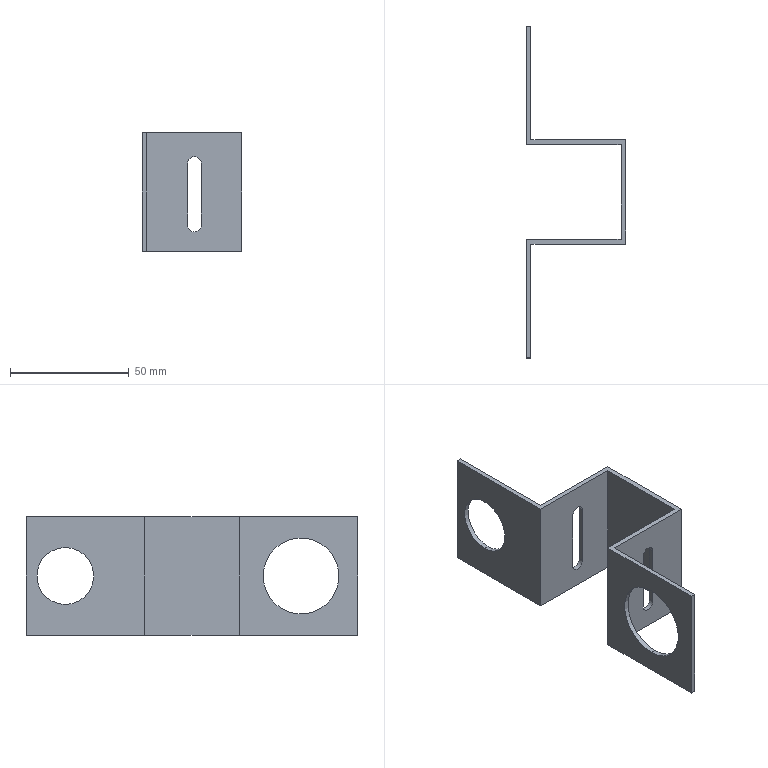Part | SolidWorks | features ICE 3, Extrusion 1 | 1 solid | 28 faces | box 42 x 140 x 50 mm | volume 18778 mm3 | plane 18 | cylinder 10 | commonest cylinder face diameters 5.797 x6 24 x2 32 x2
STEP:
#1=CARTESIAN_POINT('',(0.,33.474,37.));
#2=VERTEX_POINT('',#1);
#3=CARTESIAN_POINT('',(0.,33.474,13.));
#4=VERTEX_POINT('',#3);
#5=CARTESIAN_POINT('',(0.,33.474,25.));
#6=DIRECTION('',(1.,0.,0.));
#7=DIRECTION('',(0.,1.,0.));
#8=AXIS2_PLACEMENT_3D('',#5,#6,#7);
#9=CIRCLE('',#8,12.);
#10=EDGE_CURVE('',#2,#4,#9,.T.);
#11=ORIENTED_EDGE('',*,*,#10,.F.);
#12=CARTESIAN_POINT('',(2.,33.474,37.));
#13=VERTEX_POINT('',#12);
#14=CARTESIAN_POINT('',(-48.,33.474,37.));
#15=DIRECTION('',(1.,0.,0.));
#16=VECTOR('',#15,1000.);
#17=LINE('',#14,#16);
#18=EDGE_CURVE('',#2,#13,#17,.T.);
#19=ORIENTED_EDGE('',*,*,#18,.T.);
#20=CARTESIAN_POINT('',(2.,33.474,13.));
#21=VERTEX_POINT('',#20);
#22=CARTESIAN_POINT('',(2.,33.474,25.));
#23=DIRECTION('',(1.,0.,0.));
#24=DIRECTION('',(0.,0.,-1.));
#25=AXIS2_PLACEMENT_3D('',#22,#23,#24);
#26=CIRCLE('',#25,12.);
#27=EDGE_CURVE('',#13,#21,#26,.T.);
#28=ORIENTED_EDGE('',*,*,#27,.T.);
#29=CARTESIAN_POINT('',(-48.,33.474,13.));
#30=DIRECTION('',(1.,0.,0.));
#31=VECTOR('',#30,1000.);
#32=LINE('',#29,#31);
#33=EDGE_CURVE('',#4,#21,#32,.T.);
#34=ORIENTED_EDGE('',*,*,#33,.F.);
#35=EDGE_LOOP('',(#11,#19,#28,#34));
#36=FACE_OUTER_BOUND('',#35,.T.);
#37=CARTESIAN_POINT('',(-48.,33.474,25.));
#38=DIRECTION('',(1.,0.,0.));
#39=DIRECTION('',(0.,0.,-1.));
#40=AXIS2_PLACEMENT_3D('',#37,#38,#39);
#41=CYLINDRICAL_SURFACE('',#40,12.);
#42=ADVANCED_FACE('',(#36),#41,.F.);
#43=CARTESIAN_POINT('',(0.,-66.,41.));
#44=VERTEX_POINT('',#43);
#45=CARTESIAN_POINT('',(0.,-66.,9.));
#46=VERTEX_POINT('',#45);
#47=CARTESIAN_POINT('',(0.,-66.,25.));
#48=DIRECTION('',(1.,0.,0.));
#49=DIRECTION('',(0.,1.,0.));
#50=AXIS2_PLACEMENT_3D('',#47,#48,#49);
#51=CIRCLE('',#50,16.);
#52=EDGE_CURVE('',#44,#46,#51,.T.);
#53=ORIENTED_EDGE('',*,*,#52,.F.);
#54=CARTESIAN_POINT('',(2.,-66.,41.));
#55=VERTEX_POINT('',#54);
#56=CARTESIAN_POINT('',(-48.,-66.,41.));
#57=DIRECTION('',(1.,0.,0.));
#58=VECTOR('',#57,1000.);
#59=LINE('',#56,#58);
#60=EDGE_CURVE('',#44,#55,#59,.T.);
#61=ORIENTED_EDGE('',*,*,#60,.T.);
#62=CARTESIAN_POINT('',(2.,-66.,9.));
#63=VERTEX_POINT('',#62);
#64=CARTESIAN_POINT('',(2.,-66.,25.));
#65=DIRECTION('',(1.,0.,0.));
#66=DIRECTION('',(0.,0.,-1.));
#67=AXIS2_PLACEMENT_3D('',#64,#65,#66);
#68=CIRCLE('',#67,16.);
#69=EDGE_CURVE('',#55,#63,#68,.T.);
#70=ORIENTED_EDGE('',*,*,#69,.T.);
#71=CARTESIAN_POINT('',(-48.,-66.,9.));
#72=DIRECTION('',(1.,0.,0.));
#73=VECTOR('',#72,1000.);
#74=LINE('',#71,#73);
#75=EDGE_CURVE('',#46,#63,#74,.T.);
#76=ORIENTED_EDGE('',*,*,#75,.F.);
#77=EDGE_LOOP('',(#53,#61,#70,#76));
#78=FACE_OUTER_BOUND('',#77,.T.);
#79=CARTESIAN_POINT('',(-48.,-66.,25.));
#80=DIRECTION('',(1.,0.,0.));
#81=DIRECTION('',(0.,0.,-1.));
#82=AXIS2_PLACEMENT_3D('',#79,#80,#81);
#83=CYLINDRICAL_SURFACE('',#82,16.);
#84=ADVANCED_FACE('',(#78),#83,.F.);
#85=CARTESIAN_POINT('',(22.,-42.,39.928));
#86=VERTEX_POINT('',#85);
#87=CARTESIAN_POINT('',(24.898,-42.,37.029));
#88=VERTEX_POINT('',#87);
#89=CARTESIAN_POINT('',(22.,-42.,37.029));
#90=DIRECTION('',(0.,1.,0.));
#91=DIRECTION('',(0.,0.,1.));
#92=AXIS2_PLACEMENT_3D('',#89,#90,#91);
#93=CIRCLE('',#92,2.898);
#94=EDGE_CURVE('',#86,#88,#93,.T.);
#95=ORIENTED_EDGE('',*,*,#94,.F.);
#96=CARTESIAN_POINT('',(22.,-40.,39.928));
#97=VERTEX_POINT('',#96);
#98=CARTESIAN_POINT('',(22.,-48.,39.928));
#99=DIRECTION('',(0.,1.,0.));
#100=VECTOR('',#99,1000.);
#101=LINE('',#98,#100);
#102=EDGE_CURVE('',#86,#97,#101,.T.);
#103=ORIENTED_EDGE('',*,*,#102,.T.);
#104=CARTESIAN_POINT('',(24.898,-40.,37.029));
#105=VERTEX_POINT('',#104);
#106=CARTESIAN_POINT('',(22.,-40.,37.029));
#107=DIRECTION('',(0.,-1.,0.));
#108=DIRECTION('',(1.,0.,0.));
#109=AXIS2_PLACEMENT_3D('',#106,#107,#108);
#110=CIRCLE('',#109,2.898);
#111=EDGE_CURVE('',#105,#97,#110,.T.);
#112=ORIENTED_EDGE('',*,*,#111,.F.);
#113=CARTESIAN_POINT('',(24.898,-48.,37.029));
#114=DIRECTION('',(0.,1.,0.));
#115=VECTOR('',#114,1000.);
#116=LINE('',#113,#115);
#117=EDGE_CURVE('',#88,#105,#116,.T.);
#118=ORIENTED_EDGE('',*,*,#117,.F.);
#119=EDGE_LOOP('',(#95,#103,#112,#118));
#120=FACE_OUTER_BOUND('',#119,.T.);
#121=CARTESIAN_POINT('',(22.,-48.,37.029));
#122=DIRECTION('',(0.,1.,0.));
#123=DIRECTION('',(0.,0.,1.));
#124=AXIS2_PLACEMENT_3D('',#121,#122,#123);
#125=CYLINDRICAL_SURFACE('',#124,2.898);
#126=ADVANCED_FACE('',(#120),#125,.F.);
#127=CARTESIAN_POINT('',(22.,0.,39.928));
#128=VERTEX_POINT('',#127);
#129=CARTESIAN_POINT('',(24.898,0.,37.029));
#130=VERTEX_POINT('',#129);
#131=CARTESIAN_POINT('',(22.,0.,37.029));
#132=DIRECTION('',(0.,1.,0.));
#133=DIRECTION('',(0.,0.,1.));
#134=AXIS2_PLACEMENT_3D('',#131,#132,#133);
#135=CIRCLE('',#134,2.898);
#136=EDGE_CURVE('',#128,#130,#135,.T.);
#137=ORIENTED_EDGE('',*,*,#136,.F.);
#138=CARTESIAN_POINT('',(22.,2.,39.928));
#139=VERTEX_POINT('',#138);
#140=CARTESIAN_POINT('',(22.,-48.,39.928));
#141=DIRECTION('',(0.,1.,0.));
#142=VECTOR('',#141,1000.);
#143=LINE('',#140,#142);
#144=EDGE_CURVE('',#128,#139,#143,.T.);
#145=ORIENTED_EDGE('',*,*,#144,.T.);
#146=CARTESIAN_POINT('',(24.898,2.,37.029));
#147=VERTEX_POINT('',#146);
#148=CARTESIAN_POINT('',(22.,2.,37.029));
#149=DIRECTION('',(0.,1.,0.));
#150=DIRECTION('',(0.,0.,1.));
#151=AXIS2_PLACEMENT_3D('',#148,#149,#150);
#152=CIRCLE('',#151,2.898);
#153=EDGE_CURVE('',#139,#147,#152,.T.);
#154=ORIENTED_EDGE('',*,*,#153,.T.);
#155=CARTESIAN_POINT('',(24.898,-48.,37.029));
#156=DIRECTION('',(0.,1.,0.));
#157=VECTOR('',#156,1000.);
#158=LINE('',#155,#157);
#159=EDGE_CURVE('',#130,#147,#158,.T.);
#160=ORIENTED_EDGE('',*,*,#159,.F.);
#161=EDGE_LOOP('',(#137,#145,#154,#160));
#162=FACE_OUTER_BOUND('',#161,.T.);
#163=CARTESIAN_POINT('',(22.,-48.,37.029));
#164=DIRECTION('',(0.,1.,0.));
#165=DIRECTION('',(0.,0.,1.));
#166=AXIS2_PLACEMENT_3D('',#163,#164,#165);
#167=CYLINDRICAL_SURFACE('',#166,2.898);
#168=ADVANCED_FACE('',(#162),#167,.F.);
#169=CARTESIAN_POINT('',(2.,50.,0.));
#170=VERTEX_POINT('',#169);
#171=CARTESIAN_POINT('',(0.,50.,0.));
#172=VERTEX_POINT('',#171);
#173=CARTESIAN_POINT('',(0.,50.,0.));
#174=DIRECTION('',(-1.,0.,0.));
#175=VECTOR('',#174,1000.);
#176=LINE('',#173,#175);
#177=EDGE_CURVE('',#170,#172,#176,.T.);
#178=ORIENTED_EDGE('',*,*,#177,.T.);
#179=CARTESIAN_POINT('',(0.,50.,50.));
#180=VERTEX_POINT('',#179);
#181=CARTESIAN_POINT('',(0.,50.,50.));
#182=DIRECTION('',(0.,0.,-1.));
#183=VECTOR('',#182,1000.);
#184=LINE('',#181,#183);
#185=EDGE_CURVE('',#180,#172,#184,.T.);
#186=ORIENTED_EDGE('',*,*,#185,.F.);
#187=CARTESIAN_POINT('',(2.,50.,50.));
#188=VERTEX_POINT('',#187);
#189=CARTESIAN_POINT('',(0.,50.,50.));
#190=DIRECTION('',(-1.,0.,0.));
#191=VECTOR('',#190,1000.);
#192=LINE('',#189,#191);
#193=EDGE_CURVE('',#188,#180,#192,.T.);
#194=ORIENTED_EDGE('',*,*,#193,.F.);
#195=CARTESIAN_POINT('',(2.,50.,50.));
#196=DIRECTION('',(0.,0.,-1.));
#197=VECTOR('',#196,1000.);
#198=LINE('',#195,#197);
#199=EDGE_CURVE('',#188,#170,#198,.T.);
#200=ORIENTED_EDGE('',*,*,#199,.T.);
#201=EDGE_LOOP('',(#178,#186,#194,#200));
#202=FACE_OUTER_BOUND('',#201,.T.);
#203=CARTESIAN_POINT('',(0.,50.,50.));
#204=DIRECTION('',(0.,-1.,0.));
#205=DIRECTION('',(0.,0.,-1.));
#206=AXIS2_PLACEMENT_3D('',#203,#204,#205);
#207=PLANE('',#206);
#208=ADVANCED_FACE('',(#202),#207,.F.);
#209=CARTESIAN_POINT('',(0.,33.474,25.));
#210=DIRECTION('',(1.,0.,0.));
#211=DIRECTION('',(0.,1.,0.));
#212=AXIS2_PLACEMENT_3D('',#209,#210,#211);
#213=CIRCLE('',#212,12.);
#214=EDGE_CURVE('',#4,#2,#213,.T.);
#215=ORIENTED_EDGE('',*,*,#214,.T.);
#216=ORIENTED_EDGE('',*,*,#10,.T.);
#217=EDGE_LOOP('',(#215,#216));
#218=FACE_BOUND('',#217,.T.);
#219=CARTESIAN_POINT('',(0.,0.,0.));
#220=VERTEX_POINT('',#219);
#221=CARTESIAN_POINT('',(0.,50.,0.));
#222=DIRECTION('',(0.,-1.,0.));
#223=VECTOR('',#222,1000.);
#224=LINE('',#221,#223);
#225=EDGE_CURVE('',#172,#220,#224,.T.);
#226=ORIENTED_EDGE('',*,*,#225,.T.);
#227=CARTESIAN_POINT('',(0.,0.,50.));
#228=VERTEX_POINT('',#227);
#229=CARTESIAN_POINT('',(0.,0.,50.));
#230=DIRECTION('',(0.,0.,-1.));
#231=VECTOR('',#230,1000.);
#232=LINE('',#229,#231);
#233=EDGE_CURVE('',#228,#220,#232,.T.);
#234=ORIENTED_EDGE('',*,*,#233,.F.);
#235=CARTESIAN_POINT('',(0.,50.,50.));
#236=DIRECTION('',(0.,-1.,0.));
#237=VECTOR('',#236,1000.);
#238=LINE('',#235,#237);
#239=EDGE_CURVE('',#180,#228,#238,.T.);
#240=ORIENTED_EDGE('',*,*,#239,.F.);
#241=ORIENTED_EDGE('',*,*,#185,.T.);
#242=EDGE_LOOP('',(#226,#234,#240,#241));
#243=FACE_OUTER_BOUND('',#242,.T.);
#244=CARTESIAN_POINT('',(0.,50.,50.));
#245=DIRECTION('',(1.,0.,0.));
#246=DIRECTION('',(0.,1.,0.));
#247=AXIS2_PLACEMENT_3D('',#244,#245,#246);
#248=PLANE('',#247);
#249=ADVANCED_FACE('',(#218,#243),#248,.F.);
#250=CARTESIAN_POINT('',(24.898,0.,11.027));
#251=VERTEX_POINT('',#250);
#252=CARTESIAN_POINT('',(24.898,0.,50.));
#253=DIRECTION('',(0.,0.,-1.));
#254=VECTOR('',#253,1000.);
#255=LINE('',#252,#254);
#256=EDGE_CURVE('',#130,#251,#255,.T.);
#257=ORIENTED_EDGE('',*,*,#256,.T.);
#258=CARTESIAN_POINT('',(19.102,0.,11.027));
#259=VERTEX_POINT('',#258);
#260=CARTESIAN_POINT('',(22.,0.,11.027));
#261=DIRECTION('',(0.,1.,0.));
#262=DIRECTION('',(0.,0.,1.));
#263=AXIS2_PLACEMENT_3D('',#260,#261,#262);
#264=CIRCLE('',#263,2.898);
#265=EDGE_CURVE('',#251,#259,#264,.T.);
#266=ORIENTED_EDGE('',*,*,#265,.T.);
#267=CARTESIAN_POINT('',(19.102,0.,37.029));
#268=VERTEX_POINT('',#267);
#269=CARTESIAN_POINT('',(19.102,0.,50.));
#270=DIRECTION('',(0.,0.,1.));
#271=VECTOR('',#270,1000.);
#272=LINE('',#269,#271);
#273=EDGE_CURVE('',#259,#268,#272,.T.);
#274=ORIENTED_EDGE('',*,*,#273,.T.);
#275=CARTESIAN_POINT('',(22.,0.,37.029));
#276=DIRECTION('',(0.,1.,0.));
#277=DIRECTION('',(0.,0.,1.));
#278=AXIS2_PLACEMENT_3D('',#275,#276,#277);
#279=CIRCLE('',#278,2.898);
#280=EDGE_CURVE('',#268,#128,#279,.T.);
#281=ORIENTED_EDGE('',*,*,#280,.T.);
#282=ORIENTED_EDGE('',*,*,#136,.T.);
#283=EDGE_LOOP('',(#257,#266,#274,#281,#282));
#284=FACE_BOUND('',#283,.T.);
#285=CARTESIAN_POINT('',(40.,0.,0.));
#286=VERTEX_POINT('',#285);
#287=CARTESIAN_POINT('',(0.,0.,0.));
#288=DIRECTION('',(1.,0.,0.));
#289=VECTOR('',#288,1000.);
#290=LINE('',#287,#289);
#291=EDGE_CURVE('',#220,#286,#290,.T.);
#292=ORIENTED_EDGE('',*,*,#291,.T.);
#293=CARTESIAN_POINT('',(40.,0.,50.));
#294=VERTEX_POINT('',#293);
#295=CARTESIAN_POINT('',(40.,0.,50.));
#296=DIRECTION('',(0.,0.,-1.));
#297=VECTOR('',#296,1000.);
#298=LINE('',#295,#297);
#299=EDGE_CURVE('',#294,#286,#298,.T.);
#300=ORIENTED_EDGE('',*,*,#299,.F.);
#301=CARTESIAN_POINT('',(0.,0.,50.));
#302=DIRECTION('',(1.,0.,0.));
#303=VECTOR('',#302,1000.);
#304=LINE('',#301,#303);
#305=EDGE_CURVE('',#228,#294,#304,.T.);
#306=ORIENTED_EDGE('',*,*,#305,.F.);
#307=ORIENTED_EDGE('',*,*,#233,.T.);
#308=EDGE_LOOP('',(#292,#300,#306,#307));
#309=FACE_OUTER_BOUND('',#308,.T.);
#310=CARTESIAN_POINT('',(0.,0.,50.));
#311=DIRECTION('',(0.,1.,0.));
#312=DIRECTION('',(0.,0.,1.));
#313=AXIS2_PLACEMENT_3D('',#310,#311,#312);
#314=PLANE('',#313);
#315=ADVANCED_FACE('',(#284,#309),#314,.F.);
#316=CARTESIAN_POINT('',(40.,-40.,0.));
#317=VERTEX_POINT('',#316);
#318=CARTESIAN_POINT('',(40.,0.,0.));
#319=DIRECTION('',(0.,-1.,0.));
#320=VECTOR('',#319,1000.);
#321=LINE('',#318,#320);
#322=EDGE_CURVE('',#286,#317,#321,.T.);
#323=ORIENTED_EDGE('',*,*,#322,.T.);
#324=CARTESIAN_POINT('',(40.,-40.,50.));
#325=VERTEX_POINT('',#324);
#326=CARTESIAN_POINT('',(40.,-40.,50.));
#327=DIRECTION('',(0.,0.,-1.));
#328=VECTOR('',#327,1000.);
#329=LINE('',#326,#328);
#330=EDGE_CURVE('',#325,#317,#329,.T.);
#331=ORIENTED_EDGE('',*,*,#330,.F.);
#332=CARTESIAN_POINT('',(40.,0.,50.));
#333=DIRECTION('',(0.,-1.,0.));
#334=VECTOR('',#333,1000.);
#335=LINE('',#332,#334);
#336=EDGE_CURVE('',#294,#325,#335,.T.);
#337=ORIENTED_EDGE('',*,*,#336,.F.);
#338=ORIENTED_EDGE('',*,*,#299,.T.);
#339=EDGE_LOOP('',(#323,#331,#337,#338));
#340=FACE_OUTER_BOUND('',#339,.T.);
#341=CARTESIAN_POINT('',(40.,0.,50.));
#342=DIRECTION('',(1.,0.,0.));
#343=DIRECTION('',(0.,0.,-1.));
#344=AXIS2_PLACEMENT_3D('',#341,#342,#343);
#345=PLANE('',#344);
#346=ADVANCED_FACE('',(#340),#345,.F.);
#347=CARTESIAN_POINT('',(19.102,-40.,37.029));
#348=VERTEX_POINT('',#347);
#349=CARTESIAN_POINT('',(19.102,-40.,11.027));
#350=VERTEX_POINT('',#349);
#351=CARTESIAN_POINT('',(19.102,-40.,50.));
#352=DIRECTION('',(0.,0.,-1.));
#353=VECTOR('',#352,1000.);
#354=LINE('',#351,#353);
#355=EDGE_CURVE('',#348,#350,#354,.T.);
#356=ORIENTED_EDGE('',*,*,#355,.T.);
#357=CARTESIAN_POINT('',(24.898,-40.,11.027));
#358=VERTEX_POINT('',#357);
#359=CARTESIAN_POINT('',(22.,-40.,11.027));
#360=DIRECTION('',(0.,-1.,0.));
#361=DIRECTION('',(1.,0.,0.));
#362=AXIS2_PLACEMENT_3D('',#359,#360,#361);
#363=CIRCLE('',#362,2.898);
#364=EDGE_CURVE('',#350,#358,#363,.T.);
#365=ORIENTED_EDGE('',*,*,#364,.T.);
#366=CARTESIAN_POINT('',(24.898,-40.,50.));
#367=DIRECTION('',(0.,0.,1.));
#368=VECTOR('',#367,1000.);
#369=LINE('',#366,#368);
#370=EDGE_CURVE('',#358,#105,#369,.T.);
#371=ORIENTED_EDGE('',*,*,#370,.T.);
#372=ORIENTED_EDGE('',*,*,#111,.T.);
#373=CARTESIAN_POINT('',(22.,-40.,37.029));
#374=DIRECTION('',(0.,-1.,0.));
#375=DIRECTION('',(1.,0.,0.));
#376=AXIS2_PLACEMENT_3D('',#373,#374,#375);
#377=CIRCLE('',#376,2.898);
#378=EDGE_CURVE('',#97,#348,#377,.T.);
#379=ORIENTED_EDGE('',*,*,#378,.T.);
#380=EDGE_LOOP('',(#356,#365,#371,#372,#379));
#381=FACE_BOUND('',#380,.T.);
#382=CARTESIAN_POINT('',(0.,-40.,0.));
#383=VERTEX_POINT('',#382);
#384=CARTESIAN_POINT('',(40.,-40.,0.));
#385=DIRECTION('',(-1.,0.,0.));
#386=VECTOR('',#385,1000.);
#387=LINE('',#384,#386);
#388=EDGE_CURVE('',#317,#383,#387,.T.);
#389=ORIENTED_EDGE('',*,*,#388,.T.);
#390=CARTESIAN_POINT('',(0.,-40.,50.));
#391=VERTEX_POINT('',#390);
#392=CARTESIAN_POINT('',(0.,-40.,50.));
#393=DIRECTION('',(0.,0.,-1.));
#394=VECTOR('',#393,1000.);
#395=LINE('',#392,#394);
#396=EDGE_CURVE('',#391,#383,#395,.T.);
#397=ORIENTED_EDGE('',*,*,#396,.F.);
#398=CARTESIAN_POINT('',(40.,-40.,50.));
#399=DIRECTION('',(-1.,0.,0.));
#400=VECTOR('',#399,1000.);
#401=LINE('',#398,#400);
#402=EDGE_CURVE('',#325,#391,#401,.T.);
#403=ORIENTED_EDGE('',*,*,#402,.F.);
#404=ORIENTED_EDGE('',*,*,#330,.T.);
#405=EDGE_LOOP('',(#389,#397,#403,#404));
#406=FACE_OUTER_BOUND('',#405,.T.);
#407=CARTESIAN_POINT('',(40.,-40.,50.));
#408=DIRECTION('',(0.,-1.,0.));
#409=DIRECTION('',(1.,0.,0.));
#410=AXIS2_PLACEMENT_3D('',#407,#408,#409);
#411=PLANE('',#410);
#412=ADVANCED_FACE('',(#381,#406),#411,.F.);
#413=CARTESIAN_POINT('',(0.,-66.,25.));
#414=DIRECTION('',(1.,0.,0.));
#415=DIRECTION('',(0.,1.,0.));
#416=AXIS2_PLACEMENT_3D('',#413,#414,#415);
#417=CIRCLE('',#416,16.);
#418=EDGE_CURVE('',#46,#44,#417,.T.);
#419=ORIENTED_EDGE('',*,*,#418,.T.);
#420=ORIENTED_EDGE('',*,*,#52,.T.);
#421=EDGE_LOOP('',(#419,#420));
#422=FACE_BOUND('',#421,.T.);
#423=CARTESIAN_POINT('',(0.,-90.,0.));
#424=VERTEX_POINT('',#423);
#425=CARTESIAN_POINT('',(0.,-40.,0.));
#426=DIRECTION('',(0.,-1.,0.));
#427=VECTOR('',#426,1000.);
#428=LINE('',#425,#427);
#429=EDGE_CURVE('',#383,#424,#428,.T.);
#430=ORIENTED_EDGE('',*,*,#429,.T.);
#431=CARTESIAN_POINT('',(0.,-90.,50.));
#432=VERTEX_POINT('',#431);
#433=CARTESIAN_POINT('',(0.,-90.,50.));
#434=DIRECTION('',(0.,0.,-1.));
#435=VECTOR('',#434,1000.);
#436=LINE('',#433,#435);
#437=EDGE_CURVE('',#432,#424,#436,.T.);
#438=ORIENTED_EDGE('',*,*,#437,.F.);
#439=CARTESIAN_POINT('',(0.,-40.,50.));
#440=DIRECTION('',(0.,-1.,0.));
#441=VECTOR('',#440,1000.);
#442=LINE('',#439,#441);
#443=EDGE_CURVE('',#391,#432,#442,.T.);
#444=ORIENTED_EDGE('',*,*,#443,.F.);
#445=ORIENTED_EDGE('',*,*,#396,.T.);
#446=EDGE_LOOP('',(#430,#438,#444,#445));
#447=FACE_OUTER_BOUND('',#446,.T.);
#448=CARTESIAN_POINT('',(0.,-40.,50.));
#449=DIRECTION('',(1.,0.,0.));
#450=DIRECTION('',(0.,1.,0.));
#451=AXIS2_PLACEMENT_3D('',#448,#449,#450);
#452=PLANE('',#451);
#453=ADVANCED_FACE('',(#422,#447),#452,.F.);
#454=CARTESIAN_POINT('',(2.,-90.,0.));
#455=VERTEX_POINT('',#454);
#456=CARTESIAN_POINT('',(0.,-90.,0.));
#457=DIRECTION('',(1.,0.,0.));
#458=VECTOR('',#457,1000.);
#459=LINE('',#456,#458);
#460=EDGE_CURVE('',#424,#455,#459,.T.);
#461=ORIENTED_EDGE('',*,*,#460,.T.);
#462=CARTESIAN_POINT('',(2.,-90.,50.));
#463=VERTEX_POINT('',#462);
#464=CARTESIAN_POINT('',(2.,-90.,50.));
#465=DIRECTION('',(0.,0.,-1.));
#466=VECTOR('',#465,1000.);
#467=LINE('',#464,#466);
#468=EDGE_CURVE('',#463,#455,#467,.T.);
#469=ORIENTED_EDGE('',*,*,#468,.F.);
#470=CARTESIAN_POINT('',(0.,-90.,50.));
#471=DIRECTION('',(1.,0.,0.));
#472=VECTOR('',#471,1000.);
#473=LINE('',#470,#472);
#474=EDGE_CURVE('',#432,#463,#473,.T.);
#475=ORIENTED_EDGE('',*,*,#474,.F.);
#476=ORIENTED_EDGE('',*,*,#437,.T.);
#477=EDGE_LOOP('',(#461,#469,#475,#476));
#478=FACE_OUTER_BOUND('',#477,.T.);
#479=CARTESIAN_POINT('',(0.,-90.,50.));
#480=DIRECTION('',(0.,1.,0.));
#481=DIRECTION('',(0.,0.,1.));
#482=AXIS2_PLACEMENT_3D('',#479,#480,#481);
#483=PLANE('',#482);
#484=ADVANCED_FACE('',(#478),#483,.F.);
#485=CARTESIAN_POINT('',(2.,-66.,25.));
#486=DIRECTION('',(1.,0.,0.));
#487=DIRECTION('',(0.,0.,-1.));
#488=AXIS2_PLACEMENT_3D('',#485,#486,#487);
#489=CIRCLE('',#488,16.);
#490=EDGE_CURVE('',#63,#55,#489,.T.);
#491=ORIENTED_EDGE('',*,*,#490,.F.);
#492=ORIENTED_EDGE('',*,*,#69,.F.);
#493=EDGE_LOOP('',(#491,#492));
#494=FACE_BOUND('',#493,.T.);
#495=CARTESIAN_POINT('',(2.,-42.,0.));
#496=VERTEX_POINT('',#495);
#497=CARTESIAN_POINT('',(2.,-42.,0.));
#498=DIRECTION('',(0.,1.,0.));
#499=VECTOR('',#498,1000.);
#500=LINE('',#497,#499);
#501=EDGE_CURVE('',#455,#496,#500,.T.);
#502=ORIENTED_EDGE('',*,*,#501,.T.);
#503=CARTESIAN_POINT('',(2.,-42.,50.));
#504=VERTEX_POINT('',#503);
#505=CARTESIAN_POINT('',(2.,-42.,50.));
#506=DIRECTION('',(0.,0.,-1.));
#507=VECTOR('',#506,1000.);
#508=LINE('',#505,#507);
#509=EDGE_CURVE('',#504,#496,#508,.T.);
#510=ORIENTED_EDGE('',*,*,#509,.F.);
#511=CARTESIAN_POINT('',(2.,-42.,50.));
#512=DIRECTION('',(0.,1.,0.));
#513=VECTOR('',#512,1000.);
#514=LINE('',#511,#513);
#515=EDGE_CURVE('',#463,#504,#514,.T.);
#516=ORIENTED_EDGE('',*,*,#515,.F.);
#517=ORIENTED_EDGE('',*,*,#468,.T.);
#518=EDGE_LOOP('',(#502,#510,#516,#517));
#519=FACE_OUTER_BOUND('',#518,.T.);
#520=CARTESIAN_POINT('',(2.,-42.,50.));
#521=DIRECTION('',(-1.,0.,0.));
#522=DIRECTION('',(0.,0.,1.));
#523=AXIS2_PLACEMENT_3D('',#520,#521,#522);
#524=PLANE('',#523);
#525=ADVANCED_FACE('',(#494,#519),#524,.F.);
#526=CARTESIAN_POINT('',(24.898,-42.,11.027));
#527=VERTEX_POINT('',#526);
#528=CARTESIAN_POINT('',(24.898,-42.,50.));
#529=DIRECTION('',(0.,0.,-1.));
#530=VECTOR('',#529,1000.);
#531=LINE('',#528,#530);
#532=EDGE_CURVE('',#88,#527,#531,.T.);
#533=ORIENTED_EDGE('',*,*,#532,.T.);
#534=CARTESIAN_POINT('',(19.102,-42.,11.027));
#535=VERTEX_POINT('',#534);
#536=CARTESIAN_POINT('',(22.,-42.,11.027));
#537=DIRECTION('',(0.,1.,0.));
#538=DIRECTION('',(0.,0.,1.));
#539=AXIS2_PLACEMENT_3D('',#536,#537,#538);
#540=CIRCLE('',#539,2.898);
#541=EDGE_CURVE('',#527,#535,#540,.T.);
#542=ORIENTED_EDGE('',*,*,#541,.T.);
#543=CARTESIAN_POINT('',(19.102,-42.,37.029));
#544=VERTEX_POINT('',#543);
#545=CARTESIAN_POINT('',(19.102,-42.,50.));
#546=DIRECTION('',(0.,0.,1.));
#547=VECTOR('',#546,1000.);
#548=LINE('',#545,#547);
#549=EDGE_CURVE('',#535,#544,#548,.T.);
#550=ORIENTED_EDGE('',*,*,#549,.T.);
#551=CARTESIAN_POINT('',(22.,-42.,37.029));
#552=DIRECTION('',(0.,1.,0.));
#553=DIRECTION('',(0.,0.,1.));
#554=AXIS2_PLACEMENT_3D('',#551,#552,#553);
#555=CIRCLE('',#554,2.898);
#556=EDGE_CURVE('',#544,#86,#555,.T.);
#557=ORIENTED_EDGE('',*,*,#556,.T.);
#558=ORIENTED_EDGE('',*,*,#94,.T.);
#559=EDGE_LOOP('',(#533,#542,#550,#557,#558));
#560=FACE_BOUND('',#559,.T.);
#561=CARTESIAN_POINT('',(42.,-42.,0.));
#562=VERTEX_POINT('',#561);
#563=CARTESIAN_POINT('',(42.,-42.,0.));
#564=DIRECTION('',(1.,0.,0.));
#565=VECTOR('',#564,1000.);
#566=LINE('',#563,#565);
#567=EDGE_CURVE('',#496,#562,#566,.T.);
#568=ORIENTED_EDGE('',*,*,#567,.T.);
#569=CARTESIAN_POINT('',(42.,-42.,50.));
#570=VERTEX_POINT('',#569);
#571=CARTESIAN_POINT('',(42.,-42.,50.));
#572=DIRECTION('',(0.,0.,-1.));
#573=VECTOR('',#572,1000.);
#574=LINE('',#571,#573);
#575=EDGE_CURVE('',#570,#562,#574,.T.);
#576=ORIENTED_EDGE('',*,*,#575,.F.);
#577=CARTESIAN_POINT('',(42.,-42.,50.));
#578=DIRECTION('',(1.,0.,0.));
#579=VECTOR('',#578,1000.);
#580=LINE('',#577,#579);
#581=EDGE_CURVE('',#504,#570,#580,.T.);
#582=ORIENTED_EDGE('',*,*,#581,.F.);
#583=ORIENTED_EDGE('',*,*,#509,.T.);
#584=EDGE_LOOP('',(#568,#576,#582,#583));
#585=FACE_OUTER_BOUND('',#584,.T.);
#586=CARTESIAN_POINT('',(42.,-42.,50.));
#587=DIRECTION('',(0.,1.,0.));
#588=DIRECTION('',(0.,0.,1.));
#589=AXIS2_PLACEMENT_3D('',#586,#587,#588);
#590=PLANE('',#589);
#591=ADVANCED_FACE('',(#560,#585),#590,.F.);
#592=CARTESIAN_POINT('',(42.,2.,0.));
#593=VERTEX_POINT('',#592);
#594=CARTESIAN_POINT('',(42.,2.,0.));
#595=DIRECTION('',(0.,1.,0.));
#596=VECTOR('',#595,1000.);
#597=LINE('',#594,#596);
#598=EDGE_CURVE('',#562,#593,#597,.T.);
#599=ORIENTED_EDGE('',*,*,#598,.T.);
#600=CARTESIAN_POINT('',(42.,2.,50.));
#601=VERTEX_POINT('',#600);
#602=CARTESIAN_POINT('',(42.,2.,50.));
#603=DIRECTION('',(0.,0.,-1.));
#604=VECTOR('',#603,1000.);
#605=LINE('',#602,#604);
#606=EDGE_CURVE('',#601,#593,#605,.T.);
#607=ORIENTED_EDGE('',*,*,#606,.F.);
#608=CARTESIAN_POINT('',(42.,2.,50.));
#609=DIRECTION('',(0.,1.,0.));
#610=VECTOR('',#609,1000.);
#611=LINE('',#608,#610);
#612=EDGE_CURVE('',#570,#601,#611,.T.);
#613=ORIENTED_EDGE('',*,*,#612,.F.);
#614=ORIENTED_EDGE('',*,*,#575,.T.);
#615=EDGE_LOOP('',(#599,#607,#613,#614));
#616=FACE_OUTER_BOUND('',#615,.T.);
#617=CARTESIAN_POINT('',(42.,2.,50.));
#618=DIRECTION('',(-1.,0.,0.));
#619=DIRECTION('',(0.,0.,1.));
#620=AXIS2_PLACEMENT_3D('',#617,#618,#619);
#621=PLANE('',#620);
#622=ADVANCED_FACE('',(#616),#621,.F.);
#623=CARTESIAN_POINT('',(19.102,2.,11.027));
#624=VERTEX_POINT('',#623);
#625=CARTESIAN_POINT('',(19.102,2.,37.029));
#626=VERTEX_POINT('',#625);
#627=CARTESIAN_POINT('',(19.102,2.,11.027));
#628=DIRECTION('',(0.,0.,1.));
#629=VECTOR('',#628,1000.);
#630=LINE('',#627,#629);
#631=EDGE_CURVE('',#624,#626,#630,.T.);
#632=ORIENTED_EDGE('',*,*,#631,.F.);
#633=CARTESIAN_POINT('',(24.898,2.,11.027));
#634=VERTEX_POINT('',#633);
#635=CARTESIAN_POINT('',(22.,2.,11.027));
#636=DIRECTION('',(0.,1.,0.));
#637=DIRECTION('',(0.,0.,1.));
#638=AXIS2_PLACEMENT_3D('',#635,#636,#637);
#639=CIRCLE('',#638,2.898);
#640=EDGE_CURVE('',#634,#624,#639,.T.);
#641=ORIENTED_EDGE('',*,*,#640,.F.);
#642=CARTESIAN_POINT('',(24.898,2.,11.027));
#643=DIRECTION('',(0.,0.,-1.));
#644=VECTOR('',#643,1000.);
#645=LINE('',#642,#644);
#646=EDGE_CURVE('',#147,#634,#645,.T.);
#647=ORIENTED_EDGE('',*,*,#646,.F.);
#648=ORIENTED_EDGE('',*,*,#153,.F.);
#649=CARTESIAN_POINT('',(22.,2.,37.029));
#650=DIRECTION('',(0.,1.,0.));
#651=DIRECTION('',(0.,0.,1.));
#652=AXIS2_PLACEMENT_3D('',#649,#650,#651);
#653=CIRCLE('',#652,2.898);
#654=EDGE_CURVE('',#626,#139,#653,.T.);
#655=ORIENTED_EDGE('',*,*,#654,.F.);
#656=EDGE_LOOP('',(#632,#641,#647,#648,#655));
#657=FACE_BOUND('',#656,.T.);
#658=CARTESIAN_POINT('',(2.,2.,0.));
#659=VERTEX_POINT('',#658);
#660=CARTESIAN_POINT('',(2.,2.,0.));
#661=DIRECTION('',(-1.,0.,0.));
#662=VECTOR('',#661,1000.);
#663=LINE('',#660,#662);
#664=EDGE_CURVE('',#593,#659,#663,.T.);
#665=ORIENTED_EDGE('',*,*,#664,.T.);
#666=CARTESIAN_POINT('',(2.,2.,50.));
#667=VERTEX_POINT('',#666);
#668=CARTESIAN_POINT('',(2.,2.,50.));
#669=DIRECTION('',(0.,0.,-1.));
#670=VECTOR('',#669,1000.);
#671=LINE('',#668,#670);
#672=EDGE_CURVE('',#667,#659,#671,.T.);
#673=ORIENTED_EDGE('',*,*,#672,.F.);
#674=CARTESIAN_POINT('',(2.,2.,50.));
#675=DIRECTION('',(-1.,0.,0.));
#676=VECTOR('',#675,1000.);
#677=LINE('',#674,#676);
#678=EDGE_CURVE('',#601,#667,#677,.T.);
#679=ORIENTED_EDGE('',*,*,#678,.F.);
#680=ORIENTED_EDGE('',*,*,#606,.T.);
#681=EDGE_LOOP('',(#665,#673,#679,#680));
#682=FACE_OUTER_BOUND('',#681,.T.);
#683=CARTESIAN_POINT('',(2.,2.,50.));
#684=DIRECTION('',(0.,-1.,0.));
#685=DIRECTION('',(0.,0.,-1.));
#686=AXIS2_PLACEMENT_3D('',#683,#684,#685);
#687=PLANE('',#686);
#688=ADVANCED_FACE('',(#657,#682),#687,.F.);
#689=CARTESIAN_POINT('',(2.,33.474,25.));
#690=DIRECTION('',(1.,0.,0.));
#691=DIRECTION('',(0.,0.,-1.));
#692=AXIS2_PLACEMENT_3D('',#689,#690,#691);
#693=CIRCLE('',#692,12.);
#694=EDGE_CURVE('',#21,#13,#693,.T.);
#695=ORIENTED_EDGE('',*,*,#694,.F.);
#696=ORIENTED_EDGE('',*,*,#27,.F.);
#697=EDGE_LOOP('',(#695,#696));
#698=FACE_BOUND('',#697,.T.);
#699=CARTESIAN_POINT('',(2.,50.,0.));
#700=DIRECTION('',(0.,1.,0.));
#701=VECTOR('',#700,1000.);
#702=LINE('',#699,#701);
#703=EDGE_CURVE('',#659,#170,#702,.T.);
#704=ORIENTED_EDGE('',*,*,#703,.T.);
#705=ORIENTED_EDGE('',*,*,#199,.F.);
#706=CARTESIAN_POINT('',(2.,50.,50.));
#707=DIRECTION('',(0.,1.,0.));
#708=VECTOR('',#707,1000.);
#709=LINE('',#706,#708);
#710=EDGE_CURVE('',#667,#188,#709,.T.);
#711=ORIENTED_EDGE('',*,*,#710,.F.);
#712=ORIENTED_EDGE('',*,*,#672,.T.);
#713=EDGE_LOOP('',(#704,#705,#711,#712));
#714=FACE_OUTER_BOUND('',#713,.T.);
#715=CARTESIAN_POINT('',(2.,50.,50.));
#716=DIRECTION('',(-1.,0.,0.));
#717=DIRECTION('',(0.,0.,1.));
#718=AXIS2_PLACEMENT_3D('',#715,#716,#717);
#719=PLANE('',#718);
#720=ADVANCED_FACE('',(#698,#714),#719,.F.);
#721=ORIENTED_EDGE('',*,*,#193,.T.);
#722=ORIENTED_EDGE('',*,*,#239,.T.);
#723=ORIENTED_EDGE('',*,*,#305,.T.);
#724=ORIENTED_EDGE('',*,*,#336,.T.);
#725=ORIENTED_EDGE('',*,*,#402,.T.);
#726=ORIENTED_EDGE('',*,*,#443,.T.);
#727=ORIENTED_EDGE('',*,*,#474,.T.);
#728=ORIENTED_EDGE('',*,*,#515,.T.);
#729=ORIENTED_EDGE('',*,*,#581,.T.);
#730=ORIENTED_EDGE('',*,*,#612,.T.);
#731=ORIENTED_EDGE('',*,*,#678,.T.);
#732=ORIENTED_EDGE('',*,*,#710,.T.);
#733=EDGE_LOOP('',(#721,#722,#723,#724,#725,#726,#727,#728,#729,#730,#731,#732));
#734=FACE_OUTER_BOUND('',#733,.T.);
#735=CARTESIAN_POINT('',(0.,0.,50.));
#736=DIRECTION('',(0.,0.,-1.));
#737=DIRECTION('',(-1.,0.,0.));
#738=AXIS2_PLACEMENT_3D('',#735,#736,#737);
#739=PLANE('',#738);
#740=ADVANCED_FACE('',(#734),#739,.F.);
#741=ORIENTED_EDGE('',*,*,#177,.F.);
#742=ORIENTED_EDGE('',*,*,#703,.F.);
#743=ORIENTED_EDGE('',*,*,#664,.F.);
#744=ORIENTED_EDGE('',*,*,#598,.F.);
#745=ORIENTED_EDGE('',*,*,#567,.F.);
#746=ORIENTED_EDGE('',*,*,#501,.F.);
#747=ORIENTED_EDGE('',*,*,#460,.F.);
#748=ORIENTED_EDGE('',*,*,#429,.F.);
#749=ORIENTED_EDGE('',*,*,#388,.F.);
#750=ORIENTED_EDGE('',*,*,#322,.F.);
#751=ORIENTED_EDGE('',*,*,#291,.F.);
#752=ORIENTED_EDGE('',*,*,#225,.F.);
#753=EDGE_LOOP('',(#741,#742,#743,#744,#745,#746,#747,#748,#749,#750,#751,#752));
#754=FACE_OUTER_BOUND('',#753,.T.);
#755=CARTESIAN_POINT('',(0.,0.,0.));
#756=DIRECTION('',(0.,0.,-1.));
#757=DIRECTION('',(-1.,0.,0.));
#758=AXIS2_PLACEMENT_3D('',#755,#756,#757);
#759=PLANE('',#758);
#760=ADVANCED_FACE('',(#754),#759,.T.);
#761=CARTESIAN_POINT('',(19.102,-48.,11.027));
#762=DIRECTION('',(0.,1.,0.));
#763=VECTOR('',#762,1000.);
#764=LINE('',#761,#763);
#765=EDGE_CURVE('',#259,#624,#764,.T.);
#766=ORIENTED_EDGE('',*,*,#765,.T.);
#767=ORIENTED_EDGE('',*,*,#631,.T.);
#768=CARTESIAN_POINT('',(19.102,-48.,37.029));
#769=DIRECTION('',(0.,1.,0.));
#770=VECTOR('',#769,1000.);
#771=LINE('',#768,#770);
#772=EDGE_CURVE('',#268,#626,#771,.T.);
#773=ORIENTED_EDGE('',*,*,#772,.F.);
#774=ORIENTED_EDGE('',*,*,#273,.F.);
#775=EDGE_LOOP('',(#766,#767,#773,#774));
#776=FACE_OUTER_BOUND('',#775,.T.);
#777=CARTESIAN_POINT('',(19.102,-48.,11.027));
#778=DIRECTION('',(-1.,0.,0.));
#779=DIRECTION('',(0.,0.,1.));
#780=AXIS2_PLACEMENT_3D('',#777,#778,#779);
#781=PLANE('',#780);
#782=ADVANCED_FACE('',(#776),#781,.F.);
#783=ORIENTED_EDGE('',*,*,#144,.F.);
#784=ORIENTED_EDGE('',*,*,#280,.F.);
#785=ORIENTED_EDGE('',*,*,#772,.T.);
#786=ORIENTED_EDGE('',*,*,#654,.T.);
#787=EDGE_LOOP('',(#783,#784,#785,#786));
#788=FACE_OUTER_BOUND('',#787,.T.);
#789=CARTESIAN_POINT('',(22.,-48.,37.029));
#790=DIRECTION('',(0.,1.,0.));
#791=DIRECTION('',(0.,0.,1.));
#792=AXIS2_PLACEMENT_3D('',#789,#790,#791);
#793=CYLINDRICAL_SURFACE('',#792,2.898);
#794=ADVANCED_FACE('',(#788),#793,.F.);
#795=ORIENTED_EDGE('',*,*,#159,.T.);
#796=ORIENTED_EDGE('',*,*,#646,.T.);
#797=CARTESIAN_POINT('',(24.898,-48.,11.027));
#798=DIRECTION('',(0.,1.,0.));
#799=VECTOR('',#798,1000.);
#800=LINE('',#797,#799);
#801=EDGE_CURVE('',#251,#634,#800,.T.);
#802=ORIENTED_EDGE('',*,*,#801,.F.);
#803=ORIENTED_EDGE('',*,*,#256,.F.);
#804=EDGE_LOOP('',(#795,#796,#802,#803));
#805=FACE_OUTER_BOUND('',#804,.T.);
#806=CARTESIAN_POINT('',(24.898,-48.,11.027));
#807=DIRECTION('',(1.,0.,0.));
#808=DIRECTION('',(0.,0.,-1.));
#809=AXIS2_PLACEMENT_3D('',#806,#807,#808);
#810=PLANE('',#809);
#811=ADVANCED_FACE('',(#805),#810,.F.);
#812=ORIENTED_EDGE('',*,*,#801,.T.);
#813=ORIENTED_EDGE('',*,*,#640,.T.);
#814=ORIENTED_EDGE('',*,*,#765,.F.);
#815=ORIENTED_EDGE('',*,*,#265,.F.);
#816=EDGE_LOOP('',(#812,#813,#814,#815));
#817=FACE_OUTER_BOUND('',#816,.T.);
#818=CARTESIAN_POINT('',(22.,-48.,11.027));
#819=DIRECTION('',(0.,1.,0.));
#820=DIRECTION('',(0.,0.,1.));
#821=AXIS2_PLACEMENT_3D('',#818,#819,#820);
#822=CYLINDRICAL_SURFACE('',#821,2.898);
#823=ADVANCED_FACE('',(#817),#822,.F.);
#824=CARTESIAN_POINT('',(19.102,-48.,11.027));
#825=DIRECTION('',(0.,1.,0.));
#826=VECTOR('',#825,1000.);
#827=LINE('',#824,#826);
#828=EDGE_CURVE('',#535,#350,#827,.T.);
#829=ORIENTED_EDGE('',*,*,#828,.F.);
#830=ORIENTED_EDGE('',*,*,#541,.F.);
#831=CARTESIAN_POINT('',(24.898,-48.,11.027));
#832=DIRECTION('',(0.,1.,0.));
#833=VECTOR('',#832,1000.);
#834=LINE('',#831,#833);
#835=EDGE_CURVE('',#527,#358,#834,.T.);
#836=ORIENTED_EDGE('',*,*,#835,.T.);
#837=ORIENTED_EDGE('',*,*,#364,.F.);
#838=EDGE_LOOP('',(#829,#830,#836,#837));
#839=FACE_OUTER_BOUND('',#838,.T.);
#840=CARTESIAN_POINT('',(22.,-48.,11.027));
#841=DIRECTION('',(0.,1.,0.));
#842=DIRECTION('',(0.,0.,1.));
#843=AXIS2_PLACEMENT_3D('',#840,#841,#842);
#844=CYLINDRICAL_SURFACE('',#843,2.898);
#845=ADVANCED_FACE('',(#839),#844,.F.);
#846=ORIENTED_EDGE('',*,*,#835,.F.);
#847=ORIENTED_EDGE('',*,*,#532,.F.);
#848=ORIENTED_EDGE('',*,*,#117,.T.);
#849=ORIENTED_EDGE('',*,*,#370,.F.);
#850=EDGE_LOOP('',(#846,#847,#848,#849));
#851=FACE_OUTER_BOUND('',#850,.T.);
#852=CARTESIAN_POINT('',(24.898,-48.,11.027));
#853=DIRECTION('',(1.,0.,0.));
#854=DIRECTION('',(0.,0.,-1.));
#855=AXIS2_PLACEMENT_3D('',#852,#853,#854);
#856=PLANE('',#855);
#857=ADVANCED_FACE('',(#851),#856,.F.);
#858=ORIENTED_EDGE('',*,*,#102,.F.);
#859=ORIENTED_EDGE('',*,*,#556,.F.);
#860=CARTESIAN_POINT('',(19.102,-48.,37.029));
#861=DIRECTION('',(0.,1.,0.));
#862=VECTOR('',#861,1000.);
#863=LINE('',#860,#862);
#864=EDGE_CURVE('',#544,#348,#863,.T.);
#865=ORIENTED_EDGE('',*,*,#864,.T.);
#866=ORIENTED_EDGE('',*,*,#378,.F.);
#867=EDGE_LOOP('',(#858,#859,#865,#866));
#868=FACE_OUTER_BOUND('',#867,.T.);
#869=CARTESIAN_POINT('',(22.,-48.,37.029));
#870=DIRECTION('',(0.,1.,0.));
#871=DIRECTION('',(0.,0.,1.));
#872=AXIS2_PLACEMENT_3D('',#869,#870,#871);
#873=CYLINDRICAL_SURFACE('',#872,2.898);
#874=ADVANCED_FACE('',(#868),#873,.F.);
#875=ORIENTED_EDGE('',*,*,#864,.F.);
#876=ORIENTED_EDGE('',*,*,#549,.F.);
#877=ORIENTED_EDGE('',*,*,#828,.T.);
#878=ORIENTED_EDGE('',*,*,#355,.F.);
#879=EDGE_LOOP('',(#875,#876,#877,#878));
#880=FACE_OUTER_BOUND('',#879,.T.);
#881=CARTESIAN_POINT('',(19.102,-48.,11.027));
#882=DIRECTION('',(-1.,0.,0.));
#883=DIRECTION('',(0.,0.,1.));
#884=AXIS2_PLACEMENT_3D('',#881,#882,#883);
#885=PLANE('',#884);
#886=ADVANCED_FACE('',(#880),#885,.F.);
#887=ORIENTED_EDGE('',*,*,#60,.F.);
#888=ORIENTED_EDGE('',*,*,#418,.F.);
#889=ORIENTED_EDGE('',*,*,#75,.T.);
#890=ORIENTED_EDGE('',*,*,#490,.T.);
#891=EDGE_LOOP('',(#887,#888,#889,#890));
#892=FACE_OUTER_BOUND('',#891,.T.);
#893=CARTESIAN_POINT('',(-48.,-66.,25.));
#894=DIRECTION('',(1.,0.,0.));
#895=DIRECTION('',(0.,0.,-1.));
#896=AXIS2_PLACEMENT_3D('',#893,#894,#895);
#897=CYLINDRICAL_SURFACE('',#896,16.);
#898=ADVANCED_FACE('',(#892),#897,.F.);
#899=ORIENTED_EDGE('',*,*,#18,.F.);
#900=ORIENTED_EDGE('',*,*,#214,.F.);
#901=ORIENTED_EDGE('',*,*,#33,.T.);
#902=ORIENTED_EDGE('',*,*,#694,.T.);
#903=EDGE_LOOP('',(#899,#900,#901,#902));
#904=FACE_OUTER_BOUND('',#903,.T.);
#905=CARTESIAN_POINT('',(-48.,33.474,25.));
#906=DIRECTION('',(1.,0.,0.));
#907=DIRECTION('',(0.,0.,-1.));
#908=AXIS2_PLACEMENT_3D('',#905,#906,#907);
#909=CYLINDRICAL_SURFACE('',#908,12.);
#910=ADVANCED_FACE('',(#904),#909,.F.);
#911=CLOSED_SHELL('',(#42,#84,#126,#168,#208,#249,#315,#346,#412,#453,#484,#525,#591,#622,#688,#720,#740,#760,#782,#794,#811,#823,#845,#857,#874,#886,#898,#910));
#912=MANIFOLD_SOLID_BREP('',#911);
#913=CARTESIAN_POINT('',(0.,0.,0.));
#914=DIRECTION('',(0.,0.,1.));
#915=DIRECTION('',(1.,0.,0.));
#916=AXIS2_PLACEMENT_3D('',#913,#914,#915);
#917=(LENGTH_UNIT()NAMED_UNIT(*)SI_UNIT(.MILLI.,.METRE.));
#918=UNCERTAINTY_MEASURE_WITH_UNIT(LENGTH_MEASURE(0.00001),#917,'','');
#919=(NAMED_UNIT(*)PLANE_ANGLE_UNIT()SI_UNIT($,.RADIAN.));
#920=(NAMED_UNIT(*)SI_UNIT($,.STERADIAN.)SOLID_ANGLE_UNIT());
#921=(GEOMETRIC_REPRESENTATION_CONTEXT(3)GLOBAL_UNCERTAINTY_ASSIGNED_CONTEXT((#918))GLOBAL_UNIT_ASSIGNED_CONTEXT((#917,#919,#920))REPRESENTATION_CONTEXT('',''));
#922=ADVANCED_BREP_SHAPE_REPRESENTATION('',(#912,#916),#921);